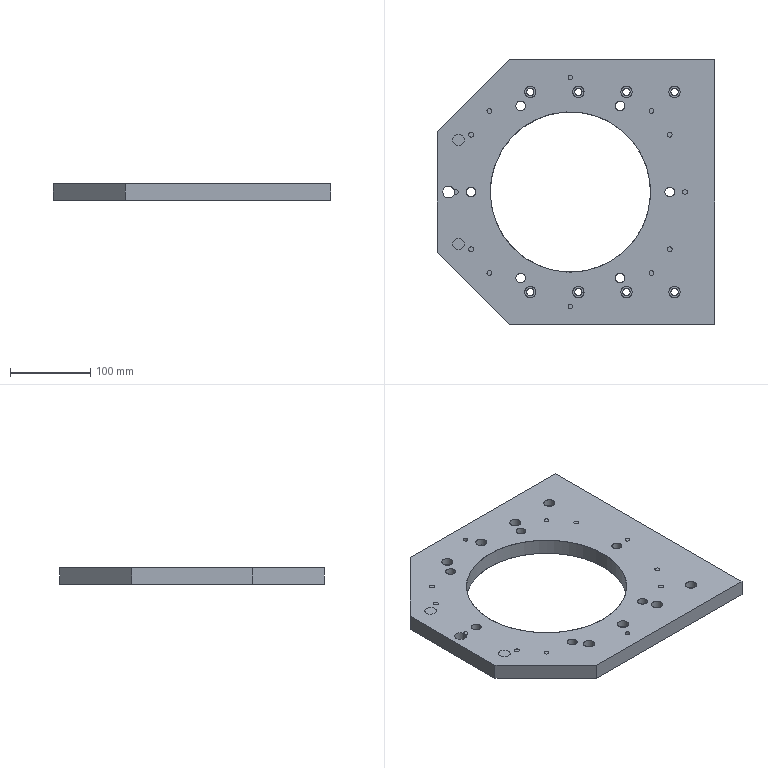NC program | NX | posted with a generic post | part box 346 x 330 x 20 mm
Lines 1 to 96 of 28317:
N10 G17 G21 G94 G90
(DRILLING , TOOL : ZXZ)
N12 T11 M6
N14 G54
N16 G17 G0 G90 X71.5 Y-130.842 S3000 M3
N18 G43 Z70. H11
N20 G94 G81 G98 Z-1. F250. R3.
N22 X107.387 Y-69.
N24 X125. Y-57.
N26 X143. Y-7.
N28 X125. Y3.
N30 X107.387 Y55.
N32 X125. Y63.
N34 Y123.
N36 X71.5 Y116.842
N38 X0. Y117.
N40 X-71.5 Y116.842
N42 X-125. Y123.
N44 Y63.
N46 X-107.387 Y55.
N48 X-125. Y3.
N50 X-143. Y-7.
N52 X-125. Y-57.
N54 X-107.387 Y-69.
N56 X-71.5 Y-130.842
N58 X0. Y-159.
N60 Y-131.
N62 Y-7.
N64 G80
N66 G0 X0. Y-7. Z70.
N68 M5
(DRILLING_COPY , TOOL : 6.0ZT)
N70 T16 M6
N72 G54
N74 G17 G0 G90 X-143. Y-7. S2000 M3
N76 G43 Z70. H16
N78 G94 G83 G98 Z-11.803 F180. Q2. R3.
N80 X-71.5 Y-130.842
N82 X71.5
N84 X143. Y-7.
N86 X71.5 Y116.842
N88 X-71.5
N90 G80
N92 G0 X-71.5 Y116.842 Z70.
N94 M5
(DRILLING_COPY_COPY , TOOL : 9.0ZT)
N96 T19 M6
N98 G54
N100 G17 G0 G90 X125. Y123. S1000 M3
N102 G43 Z70. H19
N104 G94 G83 G98 Z-23.704 F180. Q2. R3.
N106 Y63.
N108 Y3.
N110 Y-57.
N112 X-125.
N114 Y3.
N116 Y63.
N118 Y123.
N120 G80
N122 G0 X-125. Y123. Z70.
N124 M5
(DRILLING_COPY_COPY_COPY , TOOL : 12.0ZT)
N126 T12 M6
N128 G54
N130 G17 G0 G90 X-107.387 Y-69. S1000 M3
N132 G43 Z70. H12
N134 G94 G83 G98 Z-24.605 F180. Q2. R3.
N136 Y55.
N138 X0. Y117.
N140 X107.387 Y55.
N142 Y-69.
N144 X0. Y-131.
N146 G80
N148 G0 X0. Y-131. Z70.
N150 M5
(DRILLING_COPY_COPY_COPY_COPY , TOOL : 14.5ZT)
N152 T14 M6
N154 G54
N156 G17 G0 G90 X0. Y-159. S800 M3
N158 G43 Z70. H14
N160 G94 G83 G98 Z-25.356 F180. Q2. R3.
N162 G80
N164 G0 X0. Y-159. Z70.
N166 M5